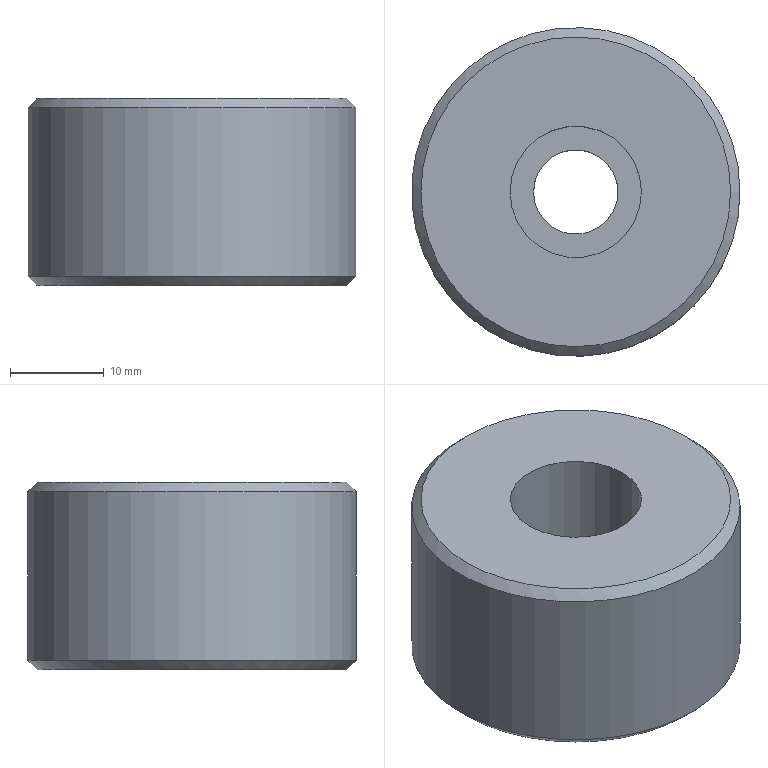Part | STEP file | 1_id1382_x_t | 1 solid | 8 faces | box 35 x 35 x 20 mm | volume 16959 mm3 | cylinder 3 | plane 3 | cone 2 | commonest cylinder face diameters 9 x1 14 x1 35 x1
STEP:
#1=CARTESIAN_POINT('',(0.,0.,0.));
#2=DIRECTION('',(0.,0.,1.));
#3=DIRECTION('',(1.,0.,0.));
#4=AXIS2_PLACEMENT_3D('',#1,#2,#3);
#5=CARTESIAN_POINT('',(-689.,0.,66.));
#6=VERTEX_POINT('',#5);
#7=CARTESIAN_POINT('',(-706.5,0.,66.));
#8=DIRECTION('',(0.,0.,1.));
#9=DIRECTION('',(1.,0.,0.));
#10=AXIS2_PLACEMENT_3D('',#7,#8,#9);
#11=CIRCLE('',#10,17.5);
#12=CARTESIAN_POINT('',(-706.5,0.,12.45));
#13=DIRECTION('',(0.,0.,1.));
#14=DIRECTION('',(-1.,0.,0.));
#15=AXIS2_PLACEMENT_3D('',#12,#13,#14);
#16=CYLINDRICAL_SURFACE('',#15,17.5);
#17=CARTESIAN_POINT('',(3.142,53.55));
#18=DIRECTION('',(1.,0.));
#19=VECTOR('',#18,1.);
#20=LINE('',#17,#19);
#21=(GEOMETRIC_REPRESENTATION_CONTEXT(2)PARAMETRIC_REPRESENTATION_CONTEXT()REPRESENTATION_CONTEXT('',''));
#22=DEFINITIONAL_REPRESENTATION('',(#20),#21);
#23=PCURVE('',#16,#22);
#24=CARTESIAN_POINT('',(-706.5,0.,65.));
#25=DIRECTION('',(0.,0.,1.));
#26=DIRECTION('',(-1.,0.,0.));
#27=AXIS2_PLACEMENT_3D('',#24,#25,#26);
#28=CONICAL_SURFACE('',#27,16.5,0.7854);
#29=CARTESIAN_POINT('',(3.142,1.));
#30=DIRECTION('',(1.,0.));
#31=VECTOR('',#30,1.);
#32=LINE('',#29,#31);
#33=(GEOMETRIC_REPRESENTATION_CONTEXT(2)PARAMETRIC_REPRESENTATION_CONTEXT()REPRESENTATION_CONTEXT('',''));
#34=DEFINITIONAL_REPRESENTATION('',(#32),#33);
#35=PCURVE('',#28,#34);
#36=SURFACE_CURVE('',#11,(#23,#35),.PCURVE_S1.);
#37=EDGE_CURVE('',#6,#6,#36,.T.);
#38=ORIENTED_EDGE('',*,*,#37,.T.);
#39=CARTESIAN_POINT('',(-689.,0.,84.));
#40=VERTEX_POINT('',#39);
#41=CARTESIAN_POINT('',(-689.,0.,66.));
#42=CARTESIAN_POINT('',(-689.,0.,84.));
#43=B_SPLINE_CURVE_WITH_KNOTS('',1,(#41,#42),.UNSPECIFIED.,.F.,.F.,(2,2),(53.55,71.55),.PIECEWISE_BEZIER_KNOTS.);
#44=CARTESIAN_POINT('',(9.425,0.));
#45=DIRECTION('',(0.,1.));
#46=VECTOR('',#45,1.);
#47=LINE('',#44,#46);
#48=(GEOMETRIC_REPRESENTATION_CONTEXT(2)PARAMETRIC_REPRESENTATION_CONTEXT()REPRESENTATION_CONTEXT('',''));
#49=DEFINITIONAL_REPRESENTATION('',(#47),#48);
#50=PCURVE('',#16,#49);
#51=CARTESIAN_POINT('',(3.142,0.));
#52=DIRECTION('',(0.,1.));
#53=VECTOR('',#52,1.);
#54=LINE('',#51,#53);
#55=(GEOMETRIC_REPRESENTATION_CONTEXT(2)PARAMETRIC_REPRESENTATION_CONTEXT()REPRESENTATION_CONTEXT('',''));
#56=DEFINITIONAL_REPRESENTATION('',(#54),#55);
#57=PCURVE('',#16,#56);
#58=SEAM_CURVE('',#43,(#50,#57),.PCURVE_S1.);
#59=EDGE_CURVE('',#6,#40,#58,.T.);
#60=ORIENTED_EDGE('',*,*,#59,.T.);
#61=CARTESIAN_POINT('',(-706.5,0.,84.));
#62=DIRECTION('',(0.,0.,-1.));
#63=DIRECTION('',(1.,0.,0.));
#64=AXIS2_PLACEMENT_3D('',#61,#62,#63);
#65=CIRCLE('',#64,17.5);
#66=CARTESIAN_POINT('',(9.425,71.55));
#67=DIRECTION('',(-1.,0.));
#68=VECTOR('',#67,1.);
#69=LINE('',#66,#68);
#70=(GEOMETRIC_REPRESENTATION_CONTEXT(2)PARAMETRIC_REPRESENTATION_CONTEXT()REPRESENTATION_CONTEXT('',''));
#71=DEFINITIONAL_REPRESENTATION('',(#69),#70);
#72=PCURVE('',#16,#71);
#73=CARTESIAN_POINT('',(-706.5,0.,84.));
#74=DIRECTION('',(0.,0.,-1.));
#75=DIRECTION('',(1.,0.,0.));
#76=AXIS2_PLACEMENT_3D('',#73,#74,#75);
#77=CONICAL_SURFACE('',#76,17.5,0.7854);
#78=CARTESIAN_POINT('',(0.,0.));
#79=DIRECTION('',(1.,0.));
#80=VECTOR('',#79,1.);
#81=LINE('',#78,#80);
#82=(GEOMETRIC_REPRESENTATION_CONTEXT(2)PARAMETRIC_REPRESENTATION_CONTEXT()REPRESENTATION_CONTEXT('',''));
#83=DEFINITIONAL_REPRESENTATION('',(#81),#82);
#84=PCURVE('',#77,#83);
#85=SURFACE_CURVE('',#65,(#72,#84),.PCURVE_S1.);
#86=EDGE_CURVE('',#40,#40,#85,.T.);
#87=ORIENTED_EDGE('',*,*,#86,.T.);
#88=ORIENTED_EDGE('',*,*,#59,.F.);
#89=EDGE_LOOP('',(#38,#60,#87,#88));
#90=FACE_BOUND('',#89,.T.);
#91=ADVANCED_FACE('',(#90),#16,.T.);
#92=CARTESIAN_POINT('',(-699.5,0.,85.));
#93=VERTEX_POINT('',#92);
#94=CARTESIAN_POINT('',(-706.5,0.,85.));
#95=DIRECTION('',(0.,0.,-1.));
#96=DIRECTION('',(1.,0.,0.));
#97=AXIS2_PLACEMENT_3D('',#94,#95,#96);
#98=CIRCLE('',#97,7.);
#99=CARTESIAN_POINT('',(-706.5,0.,52.45));
#100=DIRECTION('',(0.,0.,1.));
#101=DIRECTION('',(-1.,0.,0.));
#102=AXIS2_PLACEMENT_3D('',#99,#100,#101);
#103=CYLINDRICAL_SURFACE('',#102,7.);
#104=CARTESIAN_POINT('',(9.425,32.55));
#105=DIRECTION('',(-1.,0.));
#106=VECTOR('',#105,1.);
#107=LINE('',#104,#106);
#108=(GEOMETRIC_REPRESENTATION_CONTEXT(2)PARAMETRIC_REPRESENTATION_CONTEXT()REPRESENTATION_CONTEXT('',''));
#109=DEFINITIONAL_REPRESENTATION('',(#107),#108);
#110=PCURVE('',#103,#109);
#111=CARTESIAN_POINT('',(-706.5,0.,85.));
#112=DIRECTION('',(0.,0.,1.));
#113=DIRECTION('',(-1.,0.,0.));
#114=AXIS2_PLACEMENT_3D('',#111,#112,#113);
#115=PLANE('',#114);
#116=CARTESIAN_POINT('',(-7.,0.));
#117=CARTESIAN_POINT('',(-7.,12.124));
#118=CARTESIAN_POINT('',(3.5,6.062));
#119=CARTESIAN_POINT('',(14.,0.));
#120=CARTESIAN_POINT('',(3.5,-6.062));
#121=CARTESIAN_POINT('',(-7.,-12.124));
#122=CARTESIAN_POINT('',(-7.,0.));
#123=(BOUNDED_CURVE()B_SPLINE_CURVE(2,(#116,#117,#118,#119,#120,#121,#122),.UNSPECIFIED.,.T.,.F.)B_SPLINE_CURVE_WITH_KNOTS((1,2,2,2,2,1),(-2.094,0.,2.094,4.189,6.283,8.378),.UNSPECIFIED.)CURVE()GEOMETRIC_REPRESENTATION_ITEM()RATIONAL_B_SPLINE_CURVE((1.,0.5,1.,0.5,1.,0.5,1.))REPRESENTATION_ITEM(''));
#124=(GEOMETRIC_REPRESENTATION_CONTEXT(2)PARAMETRIC_REPRESENTATION_CONTEXT()REPRESENTATION_CONTEXT('',''));
#125=DEFINITIONAL_REPRESENTATION('',(#123),#124);
#126=PCURVE('',#115,#125);
#127=SURFACE_CURVE('',#98,(#110,#126),.PCURVE_S1.);
#128=EDGE_CURVE('',#93,#93,#127,.T.);
#129=ORIENTED_EDGE('',*,*,#128,.T.);
#130=CARTESIAN_POINT('',(-699.5,0.,75.));
#131=VERTEX_POINT('',#130);
#132=CARTESIAN_POINT('',(-699.5,0.,75.));
#133=CARTESIAN_POINT('',(-699.5,0.,85.));
#134=B_SPLINE_CURVE_WITH_KNOTS('',1,(#132,#133),.UNSPECIFIED.,.F.,.F.,(2,2),(22.55,32.55),.PIECEWISE_BEZIER_KNOTS.);
#135=CARTESIAN_POINT('',(3.142,0.));
#136=DIRECTION('',(0.,1.));
#137=VECTOR('',#136,1.);
#138=LINE('',#135,#137);
#139=(GEOMETRIC_REPRESENTATION_CONTEXT(2)PARAMETRIC_REPRESENTATION_CONTEXT()REPRESENTATION_CONTEXT('',''));
#140=DEFINITIONAL_REPRESENTATION('',(#138),#139);
#141=PCURVE('',#103,#140);
#142=CARTESIAN_POINT('',(9.425,0.));
#143=DIRECTION('',(0.,1.));
#144=VECTOR('',#143,1.);
#145=LINE('',#142,#144);
#146=(GEOMETRIC_REPRESENTATION_CONTEXT(2)PARAMETRIC_REPRESENTATION_CONTEXT()REPRESENTATION_CONTEXT('',''));
#147=DEFINITIONAL_REPRESENTATION('',(#145),#146);
#148=PCURVE('',#103,#147);
#149=SEAM_CURVE('',#134,(#141,#148),.PCURVE_S1.);
#150=EDGE_CURVE('',#131,#93,#149,.T.);
#151=ORIENTED_EDGE('',*,*,#150,.F.);
#152=CARTESIAN_POINT('',(-706.5,0.,75.));
#153=DIRECTION('',(0.,0.,-1.));
#154=DIRECTION('',(1.,0.,0.));
#155=AXIS2_PLACEMENT_3D('',#152,#153,#154);
#156=CIRCLE('',#155,7.);
#157=CARTESIAN_POINT('',(9.425,22.55));
#158=DIRECTION('',(-1.,0.));
#159=VECTOR('',#158,1.);
#160=LINE('',#157,#159);
#161=(GEOMETRIC_REPRESENTATION_CONTEXT(2)PARAMETRIC_REPRESENTATION_CONTEXT()REPRESENTATION_CONTEXT('',''));
#162=DEFINITIONAL_REPRESENTATION('',(#160),#161);
#163=PCURVE('',#103,#162);
#164=CARTESIAN_POINT('',(-706.5,0.,75.));
#165=DIRECTION('',(0.,0.,1.));
#166=DIRECTION('',(-1.,0.,0.));
#167=AXIS2_PLACEMENT_3D('',#164,#165,#166);
#168=PLANE('',#167);
#169=CARTESIAN_POINT('',(-7.,0.));
#170=CARTESIAN_POINT('',(-7.,12.124));
#171=CARTESIAN_POINT('',(3.5,6.062));
#172=CARTESIAN_POINT('',(14.,0.));
#173=CARTESIAN_POINT('',(3.5,-6.062));
#174=CARTESIAN_POINT('',(-7.,-12.124));
#175=CARTESIAN_POINT('',(-7.,0.));
#176=(BOUNDED_CURVE()B_SPLINE_CURVE(2,(#169,#170,#171,#172,#173,#174,#175),.UNSPECIFIED.,.T.,.F.)B_SPLINE_CURVE_WITH_KNOTS((1,2,2,2,2,1),(-2.094,0.,2.094,4.189,6.283,8.378),.UNSPECIFIED.)CURVE()GEOMETRIC_REPRESENTATION_ITEM()RATIONAL_B_SPLINE_CURVE((1.,0.5,1.,0.5,1.,0.5,1.))REPRESENTATION_ITEM(''));
#177=(GEOMETRIC_REPRESENTATION_CONTEXT(2)PARAMETRIC_REPRESENTATION_CONTEXT()REPRESENTATION_CONTEXT('',''));
#178=DEFINITIONAL_REPRESENTATION('',(#176),#177);
#179=PCURVE('',#168,#178);
#180=SURFACE_CURVE('',#156,(#163,#179),.PCURVE_S1.);
#181=EDGE_CURVE('',#131,#131,#180,.T.);
#182=ORIENTED_EDGE('',*,*,#181,.F.);
#183=ORIENTED_EDGE('',*,*,#150,.T.);
#184=EDGE_LOOP('',(#129,#151,#182,#183));
#185=FACE_BOUND('',#184,.F.);
#186=ADVANCED_FACE('',(#185),#103,.F.);
#187=CARTESIAN_POINT('',(-690.,0.,85.));
#188=VERTEX_POINT('',#187);
#189=CARTESIAN_POINT('',(-706.5,0.,85.));
#190=DIRECTION('',(0.,0.,1.));
#191=DIRECTION('',(1.,0.,0.));
#192=AXIS2_PLACEMENT_3D('',#189,#190,#191);
#193=CIRCLE('',#192,16.5);
#194=CARTESIAN_POINT('',(0.,0.));
#195=DIRECTION('',(-1.,0.));
#196=AXIS2_PLACEMENT_2D('',#194,#195);
#197=CIRCLE('',#196,16.5);
#198=(GEOMETRIC_REPRESENTATION_CONTEXT(2)PARAMETRIC_REPRESENTATION_CONTEXT()REPRESENTATION_CONTEXT('',''));
#199=DEFINITIONAL_REPRESENTATION('',(#197),#198);
#200=PCURVE('',#115,#199);
#201=CARTESIAN_POINT('',(6.283,-1.));
#202=DIRECTION('',(-1.,0.));
#203=VECTOR('',#202,1.);
#204=LINE('',#201,#203);
#205=(GEOMETRIC_REPRESENTATION_CONTEXT(2)PARAMETRIC_REPRESENTATION_CONTEXT()REPRESENTATION_CONTEXT('',''));
#206=DEFINITIONAL_REPRESENTATION('',(#204),#205);
#207=PCURVE('',#77,#206);
#208=SURFACE_CURVE('',#193,(#200,#207),.PCURVE_S1.);
#209=EDGE_CURVE('',#188,#188,#208,.T.);
#210=ORIENTED_EDGE('',*,*,#209,.T.);
#211=EDGE_LOOP('',(#210));
#212=FACE_BOUND('',#211,.T.);
#213=ORIENTED_EDGE('',*,*,#128,.T.);
#214=EDGE_LOOP('',(#213));
#215=FACE_BOUND('',#214,.T.);
#216=ADVANCED_FACE('',(#212,#215),#115,.T.);
#217=ORIENTED_EDGE('',*,*,#181,.F.);
#218=EDGE_LOOP('',(#217));
#219=FACE_BOUND('',#218,.T.);
#220=CARTESIAN_POINT('',(-702.,0.,75.));
#221=VERTEX_POINT('',#220);
#222=CARTESIAN_POINT('',(-706.5,0.,75.));
#223=DIRECTION('',(0.,0.,-1.));
#224=DIRECTION('',(1.,0.,0.));
#225=AXIS2_PLACEMENT_3D('',#222,#223,#224);
#226=CIRCLE('',#225,4.5);
#227=CARTESIAN_POINT('',(-4.5,0.));
#228=CARTESIAN_POINT('',(-4.5,7.794));
#229=CARTESIAN_POINT('',(2.25,3.897));
#230=CARTESIAN_POINT('',(9.,0.));
#231=CARTESIAN_POINT('',(2.25,-3.897));
#232=CARTESIAN_POINT('',(-4.5,-7.794));
#233=CARTESIAN_POINT('',(-4.5,0.));
#234=(BOUNDED_CURVE()B_SPLINE_CURVE(2,(#227,#228,#229,#230,#231,#232,#233),.UNSPECIFIED.,.T.,.F.)B_SPLINE_CURVE_WITH_KNOTS((1,2,2,2,2,1),(-2.094,0.,2.094,4.189,6.283,8.378),.UNSPECIFIED.)CURVE()GEOMETRIC_REPRESENTATION_ITEM()RATIONAL_B_SPLINE_CURVE((1.,0.5,1.,0.5,1.,0.5,1.))REPRESENTATION_ITEM(''));
#235=(GEOMETRIC_REPRESENTATION_CONTEXT(2)PARAMETRIC_REPRESENTATION_CONTEXT()REPRESENTATION_CONTEXT('',''));
#236=DEFINITIONAL_REPRESENTATION('',(#234),#235);
#237=PCURVE('',#168,#236);
#238=CARTESIAN_POINT('',(-706.5,0.,148.5));
#239=DIRECTION('',(0.,0.,-1.));
#240=DIRECTION('',(-1.,0.,0.));
#241=AXIS2_PLACEMENT_3D('',#238,#239,#240);
#242=CYLINDRICAL_SURFACE('',#241,4.5);
#243=CARTESIAN_POINT('',(3.142,73.5));
#244=DIRECTION('',(1.,0.));
#245=VECTOR('',#244,1.);
#246=LINE('',#243,#245);
#247=(GEOMETRIC_REPRESENTATION_CONTEXT(2)PARAMETRIC_REPRESENTATION_CONTEXT()REPRESENTATION_CONTEXT('',''));
#248=DEFINITIONAL_REPRESENTATION('',(#246),#247);
#249=PCURVE('',#242,#248);
#250=SURFACE_CURVE('',#226,(#237,#249),.PCURVE_S1.);
#251=EDGE_CURVE('',#221,#221,#250,.T.);
#252=ORIENTED_EDGE('',*,*,#251,.T.);
#253=EDGE_LOOP('',(#252));
#254=FACE_BOUND('',#253,.T.);
#255=ADVANCED_FACE('',(#219,#254),#168,.T.);
#256=CARTESIAN_POINT('',(-702.,0.,65.));
#257=VERTEX_POINT('',#256);
#258=CARTESIAN_POINT('',(-706.5,0.,65.));
#259=DIRECTION('',(0.,0.,-1.));
#260=DIRECTION('',(1.,0.,0.));
#261=AXIS2_PLACEMENT_3D('',#258,#259,#260);
#262=CIRCLE('',#261,4.5);
#263=CARTESIAN_POINT('',(3.142,83.5));
#264=DIRECTION('',(1.,0.));
#265=VECTOR('',#264,1.);
#266=LINE('',#263,#265);
#267=(GEOMETRIC_REPRESENTATION_CONTEXT(2)PARAMETRIC_REPRESENTATION_CONTEXT()REPRESENTATION_CONTEXT('',''));
#268=DEFINITIONAL_REPRESENTATION('',(#266),#267);
#269=PCURVE('',#242,#268);
#270=CARTESIAN_POINT('',(-394.,-130.,65.));
#271=DIRECTION('',(0.,0.,1.));
#272=DIRECTION('',(-1.,0.,0.));
#273=AXIS2_PLACEMENT_3D('',#270,#271,#272);
#274=PLANE('',#273);
#275=CARTESIAN_POINT('',(308.,-130.));
#276=CARTESIAN_POINT('',(308.,-122.206));
#277=CARTESIAN_POINT('',(314.75,-126.103));
#278=CARTESIAN_POINT('',(321.5,-130.));
#279=CARTESIAN_POINT('',(314.75,-133.897));
#280=CARTESIAN_POINT('',(308.,-137.794));
#281=CARTESIAN_POINT('',(308.,-130.));
#282=(BOUNDED_CURVE()B_SPLINE_CURVE(2,(#275,#276,#277,#278,#279,#280,#281),.UNSPECIFIED.,.T.,.F.)B_SPLINE_CURVE_WITH_KNOTS((1,2,2,2,2,1),(-2.094,0.,2.094,4.189,6.283,8.378),.UNSPECIFIED.)CURVE()GEOMETRIC_REPRESENTATION_ITEM()RATIONAL_B_SPLINE_CURVE((1.,0.5,1.,0.5,1.,0.5,1.))REPRESENTATION_ITEM(''));
#283=(GEOMETRIC_REPRESENTATION_CONTEXT(2)PARAMETRIC_REPRESENTATION_CONTEXT()REPRESENTATION_CONTEXT('',''));
#284=DEFINITIONAL_REPRESENTATION('',(#282),#283);
#285=PCURVE('',#274,#284);
#286=SURFACE_CURVE('',#262,(#269,#285),.PCURVE_S1.);
#287=EDGE_CURVE('',#257,#257,#286,.T.);
#288=ORIENTED_EDGE('',*,*,#287,.F.);
#289=CARTESIAN_POINT('',(-702.,0.,75.));
#290=CARTESIAN_POINT('',(-702.,0.,65.));
#291=B_SPLINE_CURVE_WITH_KNOTS('',1,(#289,#290),.UNSPECIFIED.,.F.,.F.,(2,2),(73.5,83.5),.PIECEWISE_BEZIER_KNOTS.);
#292=CARTESIAN_POINT('',(3.142,0.));
#293=DIRECTION('',(0.,1.));
#294=VECTOR('',#293,1.);
#295=LINE('',#292,#294);
#296=(GEOMETRIC_REPRESENTATION_CONTEXT(2)PARAMETRIC_REPRESENTATION_CONTEXT()REPRESENTATION_CONTEXT('',''));
#297=DEFINITIONAL_REPRESENTATION('',(#295),#296);
#298=PCURVE('',#242,#297);
#299=CARTESIAN_POINT('',(9.425,0.));
#300=DIRECTION('',(0.,1.));
#301=VECTOR('',#300,1.);
#302=LINE('',#299,#301);
#303=(GEOMETRIC_REPRESENTATION_CONTEXT(2)PARAMETRIC_REPRESENTATION_CONTEXT()REPRESENTATION_CONTEXT('',''));
#304=DEFINITIONAL_REPRESENTATION('',(#302),#303);
#305=PCURVE('',#242,#304);
#306=SEAM_CURVE('',#291,(#298,#305),.PCURVE_S1.);
#307=EDGE_CURVE('',#221,#257,#306,.T.);
#308=ORIENTED_EDGE('',*,*,#307,.F.);
#309=ORIENTED_EDGE('',*,*,#251,.T.);
#310=ORIENTED_EDGE('',*,*,#307,.T.);
#311=EDGE_LOOP('',(#288,#308,#309,#310));
#312=FACE_BOUND('',#311,.F.);
#313=ADVANCED_FACE('',(#312),#242,.F.);
#314=CARTESIAN_POINT('',(-690.,0.,65.));
#315=VERTEX_POINT('',#314);
#316=CARTESIAN_POINT('',(-706.5,0.,65.));
#317=DIRECTION('',(0.,0.,-1.));
#318=DIRECTION('',(1.,0.,0.));
#319=AXIS2_PLACEMENT_3D('',#316,#317,#318);
#320=CIRCLE('',#319,16.5);
#321=CARTESIAN_POINT('',(296.,-130.));
#322=CARTESIAN_POINT('',(296.,-101.421));
#323=CARTESIAN_POINT('',(320.75,-115.711));
#324=CARTESIAN_POINT('',(345.5,-130.));
#325=CARTESIAN_POINT('',(320.75,-144.289));
#326=CARTESIAN_POINT('',(296.,-158.579));
#327=CARTESIAN_POINT('',(296.,-130.));
#328=(BOUNDED_CURVE()B_SPLINE_CURVE(2,(#321,#322,#323,#324,#325,#326,#327),.UNSPECIFIED.,.T.,.F.)B_SPLINE_CURVE_WITH_KNOTS((1,2,2,2,2,1),(-2.094,0.,2.094,4.189,6.283,8.378),.UNSPECIFIED.)CURVE()GEOMETRIC_REPRESENTATION_ITEM()RATIONAL_B_SPLINE_CURVE((1.,0.5,1.,0.5,1.,0.5,1.))REPRESENTATION_ITEM(''));
#329=(GEOMETRIC_REPRESENTATION_CONTEXT(2)PARAMETRIC_REPRESENTATION_CONTEXT()REPRESENTATION_CONTEXT('',''));
#330=DEFINITIONAL_REPRESENTATION('',(#328),#329);
#331=PCURVE('',#274,#330);
#332=CARTESIAN_POINT('',(9.425,0.));
#333=DIRECTION('',(-1.,0.));
#334=VECTOR('',#333,1.);
#335=LINE('',#332,#334);
#336=(GEOMETRIC_REPRESENTATION_CONTEXT(2)PARAMETRIC_REPRESENTATION_CONTEXT()REPRESENTATION_CONTEXT('',''));
#337=DEFINITIONAL_REPRESENTATION('',(#335),#336);
#338=PCURVE('',#28,#337);
#339=SURFACE_CURVE('',#320,(#331,#338),.PCURVE_S1.);
#340=EDGE_CURVE('',#315,#315,#339,.T.);
#341=ORIENTED_EDGE('',*,*,#340,.T.);
#342=EDGE_LOOP('',(#341));
#343=FACE_BOUND('',#342,.T.);
#344=ORIENTED_EDGE('',*,*,#287,.F.);
#345=EDGE_LOOP('',(#344));
#346=FACE_BOUND('',#345,.T.);
#347=ADVANCED_FACE('',(#343,#346),#274,.F.);
#348=ORIENTED_EDGE('',*,*,#37,.F.);
#349=CARTESIAN_POINT('',(-690.,0.,65.));
#350=CARTESIAN_POINT('',(-689.,0.,66.));
#351=B_SPLINE_CURVE_WITH_KNOTS('',1,(#349,#350),.UNSPECIFIED.,.F.,.F.,(2,2),(0.,1.414),.PIECEWISE_BEZIER_KNOTS.);
#352=CARTESIAN_POINT('',(3.142,0.));
#353=DIRECTION('',(0.,1.));
#354=VECTOR('',#353,1.);
#355=LINE('',#352,#354);
#356=(GEOMETRIC_REPRESENTATION_CONTEXT(2)PARAMETRIC_REPRESENTATION_CONTEXT()REPRESENTATION_CONTEXT('',''));
#357=DEFINITIONAL_REPRESENTATION('',(#355),#356);
#358=PCURVE('',#28,#357);
#359=CARTESIAN_POINT('',(9.425,0.));
#360=DIRECTION('',(0.,1.));
#361=VECTOR('',#360,1.);
#362=LINE('',#359,#361);
#363=(GEOMETRIC_REPRESENTATION_CONTEXT(2)PARAMETRIC_REPRESENTATION_CONTEXT()REPRESENTATION_CONTEXT('',''));
#364=DEFINITIONAL_REPRESENTATION('',(#362),#363);
#365=PCURVE('',#28,#364);
#366=SEAM_CURVE('',#351,(#358,#365),.PCURVE_S1.);
#367=EDGE_CURVE('',#315,#6,#366,.T.);
#368=ORIENTED_EDGE('',*,*,#367,.F.);
#369=ORIENTED_EDGE('',*,*,#340,.F.);
#370=ORIENTED_EDGE('',*,*,#367,.T.);
#371=EDGE_LOOP('',(#348,#368,#369,#370));
#372=FACE_BOUND('',#371,.T.);
#373=ADVANCED_FACE('',(#372),#28,.T.);
#374=ORIENTED_EDGE('',*,*,#209,.F.);
#375=CARTESIAN_POINT('',(-690.,0.,85.));
#376=CARTESIAN_POINT('',(-689.,0.,84.));
#377=B_SPLINE_CURVE_WITH_KNOTS('',1,(#375,#376),.UNSPECIFIED.,.F.,.F.,(2,2),(-1.414,0.),.PIECEWISE_BEZIER_KNOTS.);
#378=CARTESIAN_POINT('',(6.283,0.));
#379=DIRECTION('',(0.,1.));
#380=VECTOR('',#379,1.);
#381=LINE('',#378,#380);
#382=(GEOMETRIC_REPRESENTATION_CONTEXT(2)PARAMETRIC_REPRESENTATION_CONTEXT()REPRESENTATION_CONTEXT('',''));
#383=DEFINITIONAL_REPRESENTATION('',(#381),#382);
#384=PCURVE('',#77,#383);
#385=CARTESIAN_POINT('',(0.,0.));
#386=DIRECTION('',(0.,1.));
#387=VECTOR('',#386,1.);
#388=LINE('',#385,#387);
#389=(GEOMETRIC_REPRESENTATION_CONTEXT(2)PARAMETRIC_REPRESENTATION_CONTEXT()REPRESENTATION_CONTEXT('',''));
#390=DEFINITIONAL_REPRESENTATION('',(#388),#389);
#391=PCURVE('',#77,#390);
#392=SEAM_CURVE('',#377,(#384,#391),.PCURVE_S1.);
#393=EDGE_CURVE('',#188,#40,#392,.T.);
#394=ORIENTED_EDGE('',*,*,#393,.T.);
#395=ORIENTED_EDGE('',*,*,#86,.F.);
#396=ORIENTED_EDGE('',*,*,#393,.F.);
#397=EDGE_LOOP('',(#374,#394,#395,#396));
#398=FACE_BOUND('',#397,.T.);
#399=ADVANCED_FACE('',(#398),#77,.T.);
#400=CLOSED_SHELL('',(#91,#186,#216,#255,#313,#347,#373,#399));
#401=MANIFOLD_SOLID_BREP('',#400);
#402=(LENGTH_UNIT()NAMED_UNIT(*)SI_UNIT(.MILLI.,.METRE.));
#403=UNCERTAINTY_MEASURE_WITH_UNIT(LENGTH_MEASURE(0.00001),#402,'','');
#404=(NAMED_UNIT(*)PLANE_ANGLE_UNIT()SI_UNIT($,.RADIAN.));
#405=(NAMED_UNIT(*)SI_UNIT($,.STERADIAN.)SOLID_ANGLE_UNIT());
#406=(GEOMETRIC_REPRESENTATION_CONTEXT(3)GLOBAL_UNCERTAINTY_ASSIGNED_CONTEXT((#403))GLOBAL_UNIT_ASSIGNED_CONTEXT((#402,#404,#405))REPRESENTATION_CONTEXT('',''));
#407=ADVANCED_BREP_SHAPE_REPRESENTATION('',(#4,#401),#406);